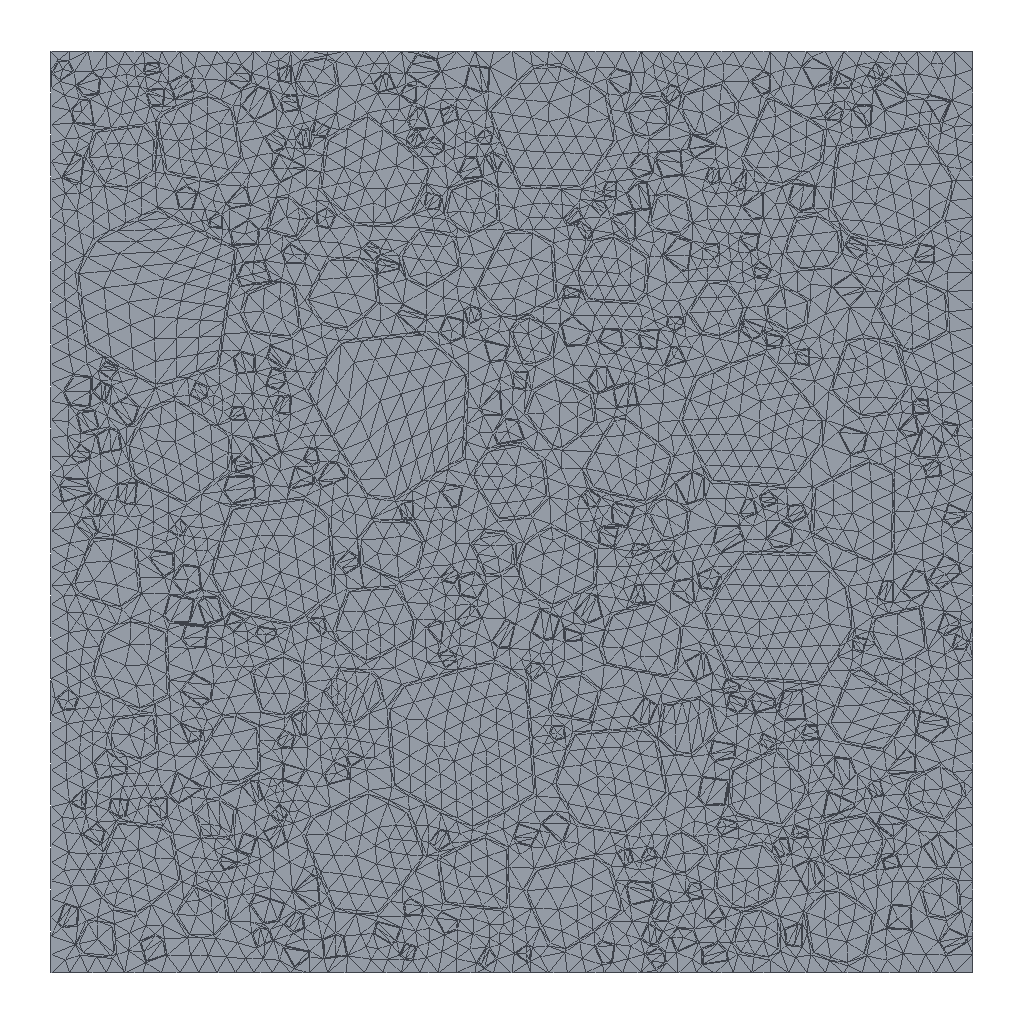Simulation study | abaqus
Set-up summary:
category,name,step,type,value,unit,region
solver,abaqus,,Abaqus/CAE 2024
units,mm-N-s-tonne (MPa),,inferred,E=60000 density=2.37e-09
analysis,Step-1,,dynamic explicit,nlgeom=True; time_period=1
mesh,nodes,,,5862
mesh,elements,,,11520
element_type,CPS3,,,11520
material,cuguliao,,E,60000
material,cuguliao,,nu,0.16
material,cuguliao,,density,2.37e-09
material,guliao-itz,,E,11375
material,guliao-itz,,nu,0.13
material,guliao-itz,,density,1.53e-09
material,guliao-itz,,behaviors,plastic; concrete damaged plasticity; concrete compression hardening; concrete tension stiffening; concrete compression damage; concrete tension damage
material,rubber,,E,100
material,rubber,,nu,0.49
material,rubber,,density,1.119e-09
material,rubber-itz,,E,6125
material,rubber-itz,,nu,0.07
material,rubber-itz,,density,8.3e-10
material,rubber-itz,,behaviors,plastic; concrete damaged plasticity; concrete compression hardening; concrete tension stiffening; concrete compression damage; concrete tension damage
material,shajiang,,E,17500
material,shajiang,,nu,0.2
material,shajiang,,density,2.36e-09
material,shajiang,,behaviors,plastic; concrete damaged plasticity; concrete compression hardening; concrete tension stiffening; concrete compression damage; concrete tension damage
section,rubber,,solid section,,,rubber
section,cuguliao,,solid section,,,guliao1
section,cuguliao,,solid section,,,guliao2
section,shajiang,,solid section,,,shajiang
section,rubber-itz,,solid section,,,rubber-itz
section,guliao-itz,,solid section,,,guliao-itz1
section,guliao-itz,,solid section,,,guliao-itz2
bc,BC-1,initial,encastre,[dofs=ENCASTRE],,_PickedSet8914
bc,BC-2,initial,fixed,"[dofs=rz,x n=2]",,Set-4
bc,BC-2,Step-1,fixed,"[dofs=rz,x n=2]",,Set-4
bc,BC-2,Step-1,displacement,-0.6 [dofs=y],,Set-4
constraint,coupling,,,1
Abaqus input file, long lists of numbers shortened:
*Heading
** Job name: deck Model name: 8mu20%-10%-Copy
** Generated by: Abaqus/CAE 2024
*Preprint, echo=NO, model=NO, history=NO, contact=NO
**
** PARTS
**
*Part, name=Part-1
*Node
      1,   96.002,   38.602
      2,   96.626,   39.924
** (5859 more lines like these left out)
*Element, type=CPS3
1,    1,    2, 3219
2, 3219,    4,    1
** (11518 more lines like these left out)
*Nset, nset=guliao-itz1
  661,  662,  663,  664,  665,  666,  667,  668,  669,  670,  671,  672,  673,  674, 1039, 1040
 1041, 1042, 1043, 1044, 1045, 1046, 1047, 1048, 1049, 1050, 1051, 1052, 1053, 1054, 1055, 1056
** (46 more lines like these left out)
*Elset, elset=guliao-itz1
  7939,  7940,  7941,  7942,  7943,  7944,  7945,  7946,  7947,  7948,  7949,  7950,  7951,  7952,  7953,  7954
  7955,  7956,  7957,  7958,  7959,  7960,  7961,  7962,  7963,  7964,  7965,  7966,  7967,  7968,  7969,  7970
** (46 more lines like these left out)
*Nset, nset=guliao1
  661,  662,  663,  664,  665,  666,  667,  668,  669,  670,  671,  672,  673,  674, 2806, 2807
 2808, 2809, 2810, 2811, 2812, 2813, 2814, 2815, 2816, 2817, 2818, 2819, 2820, 2821, 2822, 2823
** (47 more lines like these left out)
*Elset, elset=guliao1
  541,  542,  543,  544,  545,  546,  547,  548,  549,  550,  551,  552,  553,  554,  555,  556
  557,  558,  559,  560,  561,  562,  563,  564,  565,  566,  567,  568,  569,  570,  571,  572
** (70 more lines like these left out)
*Nset, nset=guliao-itz2
  675,  676,  677,  678,  679,  680,  681,  682,  683,  684,  685,  686,  687,  688,  689,  690
  691,  692,  693,  694,  695,  696,  697,  698,  699,  700,  701,  702,  703,  704,  705,  706
** (62 more lines like these left out)
*Elset, elset=guliao-itz2
  9637,  9638,  9639,  9640,  9641,  9642,  9643,  9644,  9645,  9646,  9647,  9648,  9649,  9650,  9651,  9652
  9653,  9654,  9668,  9669,  9670,  9671,  9672,  9673,  9674,  9675,  9676,  9677,  9678,  9679,  9680,  9681
** (62 more lines like these left out)
*Nset, nset=guliao2
  675,  676,  677,  678,  679,  680,  681,  682,  683,  684,  685,  686,  687,  688,  689,  690
  691,  692,  693,  694,  695,  696,  697,  698,  699,  700,  701,  702,  703,  704,  705,  706
** (42 more lines like these left out)
*Elset, elset=guliao2
   721,   722,   723,   724,   725,   726,   727,   728,   729,   730,   731,   732,   733,   734,   735,   736
   737,   738,   739,   740,   741,   742,   743,   744,   745,   746,   747,   748,   749,   750,   751,   752
** (49 more lines like these left out)
*Nset, nset=rubber-itz
    1,    2,    3,    4,    5,    6,    7,    8,    9,   10,   11,   12,   13,   14,   15,   16
   17,   18,   19,   20,   21,   22,   23,   24,   25,   26,   27,   28,   29,   30,   31,   32
** (158 more lines like these left out)
*Elset, elset=rubber-itz
  5044,  5045,  5046,  5047,  5048,  5049,  5050,  5051,  5052,  5053,  5054,  5058,  5059,  5060,  5061,  5062
  5063,  5064,  5065,  5066,  5067,  5068,  5069,  5070,  5071,  5072,  5073,  5074,  5075,  5076,  5077,  5078
** (158 more lines like these left out)
*Nset, nset=rubber
    1,    2,    3,    4,    5,    6,    7,    8,    9,   10,   11,   12,   13,   14,   15,   16
   17,   18,   19,   20,   21,   22,   23,   24,   25,   26,   27,   28,   29,   30,   31,   32
** (83 more lines like these left out)
*Elset, elset=rubber
     1,     2,     3,     4,     5,     6,     7,     8,     9,    10,    11,    12,    13,    14,    15,    16
    17,    18,    19,    20,    21,    22,    23,    24,    25,    26,    27,    28,    29,    30,    31,    32
** (58 more lines like these left out)
*Nset, nset=shajiang
  710,  711,  712,  713,  714,  715,  716,  717,  718,  719,  720,  721,  722,  723,  724,  725
  726,  727,  728,  729,  730,  731,  732,  733,  734,  735,  736,  737,  738,  739,  740,  741
** (188 more lines like these left out)
*Elset, elset=shajiang
   809,   810,   811,   812,   813,   814,   815,   816,   817,   818,   819,   820,   821,   822,   823,   824
   825,   826,   827,   828,   829,   830,   831,   832,   833,   834,   835,   836,   837,   838,   839,   840
** (267 more lines like these left out)
** Section: rubber
*Solid Section, elset=rubber, material=rubber
,
** Section: guliao
*Solid Section, elset=guliao1, material=cuguliao
,
** Section: guliao
*Solid Section, elset=guliao2, material=cuguliao
,
** Section: shajiang
*Solid Section, elset=shajiang, material=shajiang
,
** Section: rubber-itz
*Solid Section, elset=rubber-itz, material=rubber-itz
,
** Section: guliao-itz
*Solid Section, elset=guliao-itz1, material=guliao-itz
,
** Section: guliao-itz
*Solid Section, elset=guliao-itz2, material=guliao-itz
,
*End Part
**
**
** ASSEMBLY
**
*Assembly, name=Assembly
**
*Instance, name=Part-1-1, part=Part-1
*End Instance
**
*Node
      1,          50.,         82.5,           0.
*Nset, nset=Set-3, instance=Part-1-1
 2319, 2320, 4006, 4007, 4008, 4009, 4010, 4011, 4012, 4013, 4014, 4015, 4016, 4017, 4018, 4019
 4020, 4021, 4022, 4023, 4024, 4025, 4026, 4027, 4028, 4029, 4030, 4031, 4032, 4033, 4034, 4035
** (2 more lines like these left out)
*Elset, elset=Set-3, instance=Part-1-1
 1094, 1381, 1387, 1388, 1658, 1659, 1662, 1943, 1946, 2237, 2247, 2541, 2546, 2550, 2556, 3243
 3244, 3342, 3743, 3744, 3745, 3746, 3747, 3749, 3750, 3751, 3752, 3754, 3755, 3756, 3757, 3758
** (2 more lines like these left out)
*Nset, nset=Set-4
 1,
*Nset, nset=m_Set-2
 1,
*Nset, nset=rp
 1,
*Nset, nset=_PickedSet8914, internal, instance=Part-1-1
 2319, 2320, 4006, 4007, 4008, 4009, 4010, 4011, 4012, 4013, 4014, 4015, 4016, 4017, 4018, 4019
 4020, 4021, 4022, 4023, 4024, 4025, 4026, 4027, 4028, 4029, 4030, 4031, 4032, 4033, 4034, 4035
** (2 more lines like these left out)
*Elset, elset=_PickedSet8914, internal, instance=Part-1-1
 1094, 1381, 1387, 1388, 1658, 1659, 1662, 1943, 1946, 2237, 2247, 2541, 2546, 2550, 2556, 3243
 3244, 3342, 3743, 3744, 3745, 3746, 3747, 3749, 3750, 3751, 3752, 3754, 3755, 3756, 3757, 3758
** (2 more lines like these left out)
*Elset, elset=_s_Surf-1_S3, internal, instance=Part-1-1
  943,  945, 2107, 2108, 2125, 2171, 2632, 3106
*Elset, elset=_s_Surf-1_S2, internal, instance=Part-1-1
 2110, 2132, 2150, 2187, 2772, 3112, 3698, 3699, 3702, 3714, 3715, 3795, 3877, 3910, 4274, 4298
 4367, 4378, 4385, 4386, 4434, 4501, 4805, 4813, 4814, 4826, 4899
*Elset, elset=_s_Surf-1_S1, internal, instance=Part-1-1
 3694, 3695, 3696, 3697, 3701, 3703, 3704, 3705, 3706, 3707, 3709, 3710, 3712, 3716, 3717
*Surface, type=ELEMENT, name=s_Surf-1
_s_Surf-1_S3, S3
_s_Surf-1_S2, S2
_s_Surf-1_S1, S1
*Elset, elset=_s_Surf-2_S3, internal, instance=Part-1-1
  943,  945, 2107, 2108, 2125, 2171, 2632, 3106
*Elset, elset=_s_Surf-2_S2, internal, instance=Part-1-1
 2110, 2132, 2150, 2187, 2772, 3112, 3698, 3699, 3702, 3714, 3715, 3795, 3877, 3910, 4274, 4298
 4367, 4378, 4385, 4386, 4434, 4501, 4805, 4813, 4814, 4826, 4899
*Elset, elset=_s_Surf-2_S1, internal, instance=Part-1-1
 3694, 3695, 3696, 3697, 3701, 3703, 3704, 3705, 3706, 3707, 3709, 3710, 3712, 3716, 3717
*Surface, type=ELEMENT, name=s_Surf-2
_s_Surf-2_S3, S3
_s_Surf-2_S2, S2
_s_Surf-2_S1, S1
** Constraint: Constraint-1
*Coupling, constraint name=Constraint-1, ref node=m_Set-2, surface=s_Surf-2
*Kinematic
*End Assembly
*Amplitude, name=Amp-1, definition=SMOOTH STEP
             0.,              0.,             0.1,            -0.6
*Amplitude, name=Amp-2
             0.,              0.,              1.,              1.
**
** MATERIALS
**
*Material, name=cuguliao
*Density
 2.37e-09,
*Elastic
60000., 0.16
*Material, name=guliao-itz
*Density
 1.53e-09,
*Elastic
11375., 0.13
*Concrete Damaged Plasticity
38.,     0.1,    1.16, 0.6667,    0.02
*Concrete Compression Hardening
  9.36,          0.
  10.153,  1.9396e-05
  10.94,   4.381e-05
  11.726,  7.4646e-05
  12.519, 0.0001145
  13.301, 0.000166
  14.083, 0.0002365
  14.865, 0.0003448
     15.6, 0.0006593
  14.817,  0.001111
  14.036,  0.001371
  13.252,  0.001613
   12.469,  0.001853
  11.683,  0.0021
  10.899,  0.002361
  10.115,  0.002641
  9.326,  0.00295
  8.539,  0.003295
   7.758,  0.003684
  6.974,   0.00414
  6.193,  0.004685
  5.411,  0.005359
  4.629,  0.00623
  3.847,  0.007414
  3.064,  0.009156
  2.283,   0.01202
  1.502,   0.01774
 0.7219,   0.0356
 0.1559,    0.1597
*Concrete Tension Stiffening
   1.561,          0.
   1.658,   2.652e-06
   1.757,  6.2205e-06
   1.855, 1.16285e-05
      1.95, 2.87885e-05
   1.852,  7.6089e-05
   1.755, 0.0001037
   1.656, 0.0001295
   1.559, 0.000155
   1.46, 0.0001814
   1.362, 0.0002091
   1.264, 0.0002388
   1.166, 0.0002714
   1.067, 0.0003077
  0.9697, 0.0003487
  0.8718, 0.0003963
  0.7741, 0.0004531
   0.6764, 0.0005232
  0.5786, 0.0006133
  0.4809, 0.0007356
  0.383,  0.0009149
  0.2854,  0.001209
   0.1877,  0.001796
 0.09024,  0.003626
 0.01949,   0.01633
*Concrete Compression Damage
         0.,          0.
 0.002268,  1.9396e-05
 0.008194,   4.381e-05
   0.01713,  7.4646e-05
  0.029, 0.0001145
  0.04374, 0.000166
  0.06239, 0.0002365
    0.08797, 0.0003448
   0.1489, 0.0006593
   0.2157,  0.001111
   0.2486,  0.001371
   0.277,  0.001613
   0.3033,  0.001853
   0.3284,  0.0021
   0.3529,  0.002361
   0.3771,  0.002641
   0.4011,  0.00295
   0.4251,  0.003295
   0.4489,  0.003684
   0.4728,   0.00414
   0.4965,  0.004685
    0.5203,  0.005359
   0.5439,  0.00623
   0.567,  0.007414
*Concrete Tension Damage
         0.,          0.
 0.001495,   2.652e-06
 0.005916,  6.2205e-06
  0.01407, 1.16285e-05
  0.04011, 2.87885e-05
   0.1097,  7.6089e-05
   0.1492, 0.0001037
    0.1844, 0.0001295
    0.2174, 0.000155
   0.2494, 0.0001814
   0.2806, 0.0002091
   0.3113, 0.0002388
   0.3419, 0.0002714
   0.3724, 0.0003077
   0.4024, 0.0003487
   0.4325, 0.0003963
   0.4623, 0.0004531
   0.4919, 0.0005232
   0.5211, 0.0006133
   0.5496, 0.0007356
   0.5771,  0.0009149
*Material, name=rubber
*Density
 1.119e-09,
*Elastic
100., 0.49
*Material, name=rubber-itz
*Density
 8.3e-10,
*Elastic
6125., 0.07
*Concrete Damaged Plasticity
38.,     0.1,    1.16, 0.6667,    0.02
*Concrete Compression Hardening
  5.04,          0.
  5.467,  1.0444e-05
  5.891,   2.359e-05
  6.314,  4.0194e-05
  6.741,  6.1656e-05
  7.162, 8.93935e-05
  7.583, 0.0001274
  8.004, 0.0001857
      8.4, 0.000355
  7.978, 0.0005985
  7.558, 0.0007384
  7.135, 0.0008686
  6.714, 0.0009976
  6.291,  0.001131
  5.869,  0.001271
   5.447,  0.001422
  5.022,   0.001588
  4.598,  0.001774
  4.177,  0.001984
   3.755,  0.002229
  3.335,  0.002523
   2.914,  0.002886
  2.493,  0.003354
  2.072,  0.003992
  1.65,   0.00493
  1.229,  0.00647
  0.8087,  0.009555
 0.3887,   0.01917
 0.08396,   0.086
*Concrete Tension Stiffening
  0.8403,          0.
   0.893,   1.428e-06
  0.9461,  3.3495e-06
  0.9986,  6.2615e-06
      1.05, 1.55015e-05
  0.9973,  4.0971e-05
  0.9447, 5.58355e-05
   0.8919, 6.97165e-05
  0.8393, 8.34715e-05
  0.7864, 9.76675e-05
  0.7336, 0.0001126
  0.6808, 0.0001286
  0.6277, 0.0001461
  0.5747, 0.0001657
  0.5221, 0.0001877
  0.4694, 0.0002134
  0.4168, 0.000244
    0.3642, 0.0002817
  0.3116, 0.0003302
  0.2589, 0.0003961
  0.2062,  0.0004927
  0.1537, 0.0006509
   0.1011,  0.0009673
 0.04859,  0.001952
 0.0105,  0.008795
*Concrete Compression Damage
         0.,          0.
 0.001221,  1.0444e-05
 0.004412,   2.359e-05
 0.009221,  4.0194e-05
  0.01561,  6.1656e-05
  0.02355, 8.93935e-05
   0.0336, 0.0001274
  0.04737, 0.0001857
   0.0802, 0.000355
   0.1161, 0.0005985
   0.1339, 0.0007384
   0.1492, 0.0008686
    0.1633, 0.0009976
   0.1769,  0.001131
   0.19,  0.001271
   0.203,  0.001422
   0.216,   0.001588
    0.2289,  0.001774
   0.2417,  0.001984
   0.2546,  0.002229
    0.2674,  0.002523
   0.2802,  0.002886
    0.2929,  0.003354
   0.3053,  0.003992
*Concrete Tension Damage
         0.,          0.
 0.0008048,   1.428e-06
 0.003186,  3.3495e-06
 0.007578,  6.2615e-06
  0.0216, 1.55015e-05
  0.05909,  4.0971e-05
  0.08034, 5.58355e-05
  0.0993, 6.97165e-05
   0.1171, 8.34715e-05
   0.1343, 9.76675e-05
   0.1511, 0.0001126
   0.1676, 0.0001286
   0.1841, 0.0001461
   0.2005, 0.0001657
   0.2167, 0.0001877
   0.2329, 0.0002134
    0.2489, 0.000244
    0.2649, 0.0002817
   0.2806, 0.0003302
   0.296, 0.0003961
   0.3107,  0.0004927
*Material, name=shajiang
*Density
 2.36e-09,
*Elastic
17500., 0.2
*Concrete Damaged Plasticity
38.,     0.1,    1.16, 0.6667,    0.02
*Concrete Compression Hardening
 14.401,         0.
 15.62,  2.984e-05
 16.831,   6.74e-05
 18.04, 0.0001148
 19.26, 0.0001762
 20.464, 0.0002554
 21.666, 0.0003639
 22.869, 0.0005305
     24., 0.001014
 22.795, 0.00171
 21.594, 0.00211
 20.387, 0.002482
 19.183, 0.00285
 17.974,  0.003231
 16.768, 0.003632
 15.561, 0.004063
 14.348, 0.004538
 13.136, 0.005069
 11.935, 0.005668
 10.729, 0.00637
 9.528,  0.007207
 8.325, 0.008245
 7.121, 0.009584
 5.919,   0.01141
 4.714,  0.01409
 3.512,  0.01849
 2.311,  0.0273
 1.111,  0.05478
 0.2399,   0.2457
*Concrete Tension Stiffening
 2.401,         0.
  2.551,   4.08e-06
 2.703,   9.57e-06
 2.853,  1.789e-05
      3.,  4.429e-05
 2.849, 0.0001171
 2.699, 0.0001595
 2.548, 0.0001992
 2.398, 0.0002385
 2.247, 0.000279
 2.096, 0.0003216
 1.945, 0.0003673
 1.794, 0.0004176
 1.642, 0.0004734
 1.492, 0.0005364
 1.341, 0.0006098
 1.191, 0.0006971
 1.041,  0.0008049
 0.8902, 0.0009435
 0.7398, 0.001132
 0.5893,  0.001408
 0.439, 0.00186
 0.2888,  0.002764
 0.1388, 0.005578
 0.02999,  0.02513
*Concrete Compression Damage
         0.,         0.
 0.003489,  2.984e-05
  0.01261,   6.74e-05
  0.02635, 0.0001148
  0.04461, 0.0001762
  0.0673, 0.0002554
  0.09599, 0.0003639
   0.1353, 0.0005305
   0.2291, 0.001014
   0.3318, 0.00171
   0.3825, 0.00211
   0.4262, 0.002482
   0.4665, 0.00285
   0.5053,  0.003231
   0.543, 0.003632
    0.5801, 0.004063
   0.6171, 0.004538
   0.654, 0.005069
   0.6906, 0.005668
   0.7273, 0.00637
   0.7639,  0.007207
   0.8005, 0.008245
   0.8367, 0.009584
   0.8724,   0.01141
*Concrete Tension Damage
         0.,         0.
 0.002299,   4.08e-06
 0.009102,   9.57e-06
  0.02165,  1.789e-05
  0.06171,  4.429e-05
   0.1688, 0.0001171
   0.2295, 0.0001595
   0.2837, 0.0001992
   0.3345, 0.0002385
   0.3837, 0.000279
   0.4316, 0.0003216
   0.4789, 0.0003673
   0.526, 0.0004176
   0.5728, 0.0004734
   0.6191, 0.0005364
    0.6653, 0.0006098
   0.7112, 0.0006971
   0.7568,  0.0008049
   0.8017, 0.0009435
   0.8456, 0.001132
   0.8878,  0.001408
**
** INTERACTION PROPERTIES
**
*Surface Interaction, name=IntProp-1
*Friction
 0.3,
*Surface Behavior, pressure-overclosure=HARD
**
** BOUNDARY CONDITIONS
**
** Name: BC-1 Type: Symmetry/Antisymmetry/Encastre
*Boundary
_PickedSet8914, ENCASTRE
** Name: BC-2 Type: Displacement/Rotation
*Boundary
Set-4, 1, 1
Set-4, 6, 6
** ----------------------------------------------------------------
**
** STEP: Step-1
**
*Step, name=Step-1, nlgeom=YES
*Dynamic, Explicit
, 1.
*Bulk Viscosity
0.06, 1.2
** Mass Scaling: Semi-Automatic
**               Whole Model
*Variable Mass Scaling, dt=1e-06, type=below min, frequency=1
**
** BOUNDARY CONDITIONS
**
** Name: BC-2 Type: Displacement/Rotation
*Boundary, amplitude=Amp-2
Set-4, 1, 1
Set-4, 2, 2, -0.6
Set-4, 6, 6
**
** OUTPUT REQUESTS
**
*Restart, write, number interval=1, time marks=NO
**
** FIELD OUTPUT: F-Output-1
**
*Output, field
*Node Output
CF, RF, U
*Element Output, directions=YES
DAMAGEC, DAMAGET, E, LE, MISES, PE, PEEQ, PEMAG, S, SDEG
*Contact Output
CDISP, CSTRESS
**
** HISTORY OUTPUT: H-Output-1
**
*Output, history, frequency=1
*Node Output, nset=rp
RF1, RF2, RF3, RM1, RM2, RM3, RT
*End Step
Results summary:
result,odb.job_status,,,JOB_STATUS_COMPLETED_SUCCESSFULLY,"consistent, unstated (Abaqus has no unit system)"
result,steps[0].procedure,Step-1,,"*DYNAMIC, EXPLICIT","consistent, unstated (Abaqus has no unit system)"
result,steps[0].time_period,Step-1,,1,"consistent, unstated (Abaqus has no unit system)"
result,steps[0].n_frames,Step-1,,21,"consistent, unstated (Abaqus has no unit system)"
result,steps[0].last_frame.id,Step-1,,1000000,"consistent, unstated (Abaqus has no unit system)"
result,steps[0].last_frame.value,Step-1,,1,"consistent, unstated (Abaqus has no unit system)"
result,steps[0].last_frame.description,Step-1,,Increment   1000000: Step Time =    1.000,"consistent, unstated (Abaqus has no unit system)"
result,steps[0].completed,Step-1,,True,"consistent, unstated (Abaqus has no unit system)"
result,steps[0].max_U_magnitude,Step-1,,0.9456,"consistent, unstated (Abaqus has no unit system)"
result,steps[0].max_S_mises,Step-1,,21.163,"consistent, unstated (Abaqus has no unit system)"
result,steps[0].RF_sum[1],Step-1,,-0.06544,"consistent, unstated (Abaqus has no unit system)"
result,steps[0].RF_sum[2],Step-1,,-0.1316,"consistent, unstated (Abaqus has no unit system)"
result,steps[0].diagnostic.n_increments,Step-1,,28,"consistent, unstated (Abaqus has no unit system)"